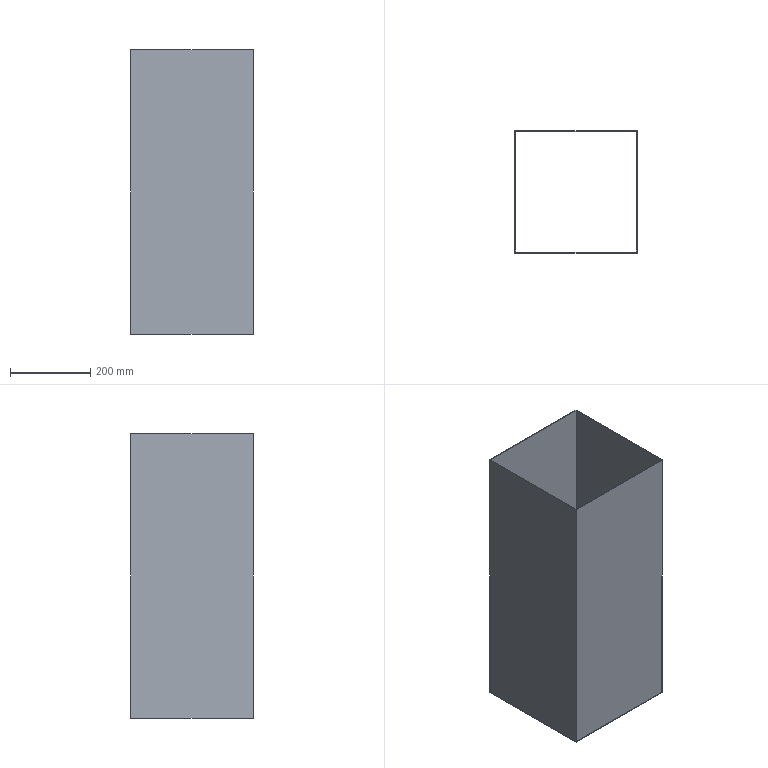Part | STEP file | Backup 2012-3-22-011 | 1 solid | 10 faces | box 304 x 304 x 708.25 mm | volume 1711132 mm3 | plane 10
STEP:
#1=CARTESIAN_POINT('',(0.,0.,0.));
#2=DIRECTION('',(0.,0.,1.));
#3=DIRECTION('',(1.,0.,0.));
#4=AXIS2_PLACEMENT_3D('',#1,#2,#3);
#5=CARTESIAN_POINT('',(-2.,2.,708.25));
#6=VERTEX_POINT('',#5);
#7=CARTESIAN_POINT('',(-2.,-302.,708.25));
#8=VERTEX_POINT('',#7);
#9=CARTESIAN_POINT('',(-2.,2.,708.25));
#10=DIRECTION('',(0.,-1.,0.));
#11=VECTOR('',#10,1.);
#12=LINE('',#9,#11);
#13=CARTESIAN_POINT('',(-2.,-302.,708.25));
#14=DIRECTION('',(0.,0.,1.));
#15=DIRECTION('',(1.,0.,0.));
#16=AXIS2_PLACEMENT_3D('',#13,#14,#15);
#17=PLANE('',#16);
#18=CARTESIAN_POINT('',(0.,304.));
#19=DIRECTION('',(0.,-1.));
#20=VECTOR('',#19,1.);
#21=LINE('',#18,#20);
#22=(GEOMETRIC_REPRESENTATION_CONTEXT(2)PARAMETRIC_REPRESENTATION_CONTEXT()REPRESENTATION_CONTEXT('',''));
#23=DEFINITIONAL_REPRESENTATION('',(#21),#22);
#24=PCURVE('',#17,#23);
#25=CARTESIAN_POINT('',(-2.,2.,708.25));
#26=DIRECTION('',(1.,0.,0.));
#27=DIRECTION('',(0.,1.,0.));
#28=AXIS2_PLACEMENT_3D('',#25,#26,#27);
#29=PLANE('',#28);
#30=CARTESIAN_POINT('',(0.,0.));
#31=DIRECTION('',(-1.,0.));
#32=VECTOR('',#31,1.);
#33=LINE('',#30,#32);
#34=(GEOMETRIC_REPRESENTATION_CONTEXT(2)PARAMETRIC_REPRESENTATION_CONTEXT()REPRESENTATION_CONTEXT('',''));
#35=DEFINITIONAL_REPRESENTATION('',(#33),#34);
#36=PCURVE('',#29,#35);
#37=SURFACE_CURVE('',#12,(#24,#36),.PCURVE_S1.);
#38=EDGE_CURVE('',#6,#8,#37,.T.);
#39=ORIENTED_EDGE('',*,*,#38,.T.);
#40=CARTESIAN_POINT('',(302.,-302.,708.25));
#41=VERTEX_POINT('',#40);
#42=CARTESIAN_POINT('',(-2.,-302.,708.25));
#43=DIRECTION('',(1.,0.,0.));
#44=VECTOR('',#43,1.);
#45=LINE('',#42,#44);
#46=CARTESIAN_POINT('',(0.,0.));
#47=DIRECTION('',(1.,0.));
#48=VECTOR('',#47,1.);
#49=LINE('',#46,#48);
#50=(GEOMETRIC_REPRESENTATION_CONTEXT(2)PARAMETRIC_REPRESENTATION_CONTEXT()REPRESENTATION_CONTEXT('',''));
#51=DEFINITIONAL_REPRESENTATION('',(#49),#50);
#52=PCURVE('',#17,#51);
#53=CARTESIAN_POINT('',(-2.,-302.,708.25));
#54=DIRECTION('',(0.,1.,0.));
#55=DIRECTION('',(0.,0.,1.));
#56=AXIS2_PLACEMENT_3D('',#53,#54,#55);
#57=PLANE('',#56);
#58=CARTESIAN_POINT('',(0.,0.));
#59=DIRECTION('',(0.,1.));
#60=VECTOR('',#59,1.);
#61=LINE('',#58,#60);
#62=(GEOMETRIC_REPRESENTATION_CONTEXT(2)PARAMETRIC_REPRESENTATION_CONTEXT()REPRESENTATION_CONTEXT('',''));
#63=DEFINITIONAL_REPRESENTATION('',(#61),#62);
#64=PCURVE('',#57,#63);
#65=SURFACE_CURVE('',#45,(#52,#64),.PCURVE_S1.);
#66=EDGE_CURVE('',#8,#41,#65,.T.);
#67=ORIENTED_EDGE('',*,*,#66,.T.);
#68=CARTESIAN_POINT('',(302.,2.,708.25));
#69=VERTEX_POINT('',#68);
#70=CARTESIAN_POINT('',(302.,2.,708.25));
#71=DIRECTION('',(0.,1.,0.));
#72=VECTOR('',#71,1.);
#73=LINE('',#70,#72);
#74=CARTESIAN_POINT('',(304.,304.));
#75=DIRECTION('',(0.,1.));
#76=VECTOR('',#75,1.);
#77=LINE('',#74,#76);
#78=(GEOMETRIC_REPRESENTATION_CONTEXT(2)PARAMETRIC_REPRESENTATION_CONTEXT()REPRESENTATION_CONTEXT('',''));
#79=DEFINITIONAL_REPRESENTATION('',(#77),#78);
#80=PCURVE('',#17,#79);
#81=CARTESIAN_POINT('',(302.,2.,708.25));
#82=DIRECTION('',(-1.,0.,0.));
#83=DIRECTION('',(0.,-1.,0.));
#84=AXIS2_PLACEMENT_3D('',#81,#82,#83);
#85=PLANE('',#84);
#86=CARTESIAN_POINT('',(0.,0.));
#87=DIRECTION('',(-1.,0.));
#88=VECTOR('',#87,1.);
#89=LINE('',#86,#88);
#90=(GEOMETRIC_REPRESENTATION_CONTEXT(2)PARAMETRIC_REPRESENTATION_CONTEXT()REPRESENTATION_CONTEXT('',''));
#91=DEFINITIONAL_REPRESENTATION('',(#89),#90);
#92=PCURVE('',#85,#91);
#93=SURFACE_CURVE('',#73,(#80,#92),.PCURVE_S1.);
#94=EDGE_CURVE('',#41,#69,#93,.T.);
#95=ORIENTED_EDGE('',*,*,#94,.T.);
#96=CARTESIAN_POINT('',(-2.,2.,708.25));
#97=DIRECTION('',(-1.,0.,0.));
#98=VECTOR('',#97,1.);
#99=LINE('',#96,#98);
#100=CARTESIAN_POINT('',(0.,304.));
#101=DIRECTION('',(-1.,0.));
#102=VECTOR('',#101,1.);
#103=LINE('',#100,#102);
#104=(GEOMETRIC_REPRESENTATION_CONTEXT(2)PARAMETRIC_REPRESENTATION_CONTEXT()REPRESENTATION_CONTEXT('',''));
#105=DEFINITIONAL_REPRESENTATION('',(#103),#104);
#106=PCURVE('',#17,#105);
#107=CARTESIAN_POINT('',(-2.,2.,708.25));
#108=DIRECTION('',(0.,-1.,0.));
#109=DIRECTION('',(0.,0.,-1.));
#110=AXIS2_PLACEMENT_3D('',#107,#108,#109);
#111=PLANE('',#110);
#112=CARTESIAN_POINT('',(0.,0.));
#113=DIRECTION('',(0.,-1.));
#114=VECTOR('',#113,1.);
#115=LINE('',#112,#114);
#116=(GEOMETRIC_REPRESENTATION_CONTEXT(2)PARAMETRIC_REPRESENTATION_CONTEXT()REPRESENTATION_CONTEXT('',''));
#117=DEFINITIONAL_REPRESENTATION('',(#115),#116);
#118=PCURVE('',#111,#117);
#119=SURFACE_CURVE('',#99,(#106,#118),.PCURVE_S1.);
#120=EDGE_CURVE('',#69,#6,#119,.T.);
#121=ORIENTED_EDGE('',*,*,#120,.T.);
#122=EDGE_LOOP('',(#39,#67,#95,#121));
#123=FACE_BOUND('',#122,.T.);
#124=CARTESIAN_POINT('',(0.,-300.,708.25));
#125=VERTEX_POINT('',#124);
#126=CARTESIAN_POINT('',(300.,-300.,708.25));
#127=VERTEX_POINT('',#126);
#128=CARTESIAN_POINT('',(0.,-300.,708.25));
#129=DIRECTION('',(1.,0.,0.));
#130=VECTOR('',#129,1.);
#131=LINE('',#128,#130);
#132=CARTESIAN_POINT('',(2.,2.));
#133=DIRECTION('',(1.,0.));
#134=VECTOR('',#133,1.);
#135=LINE('',#132,#134);
#136=(GEOMETRIC_REPRESENTATION_CONTEXT(2)PARAMETRIC_REPRESENTATION_CONTEXT()REPRESENTATION_CONTEXT('',''));
#137=DEFINITIONAL_REPRESENTATION('',(#135),#136);
#138=PCURVE('',#17,#137);
#139=CARTESIAN_POINT('',(0.,-300.,708.25));
#140=DIRECTION('',(0.,1.,0.));
#141=DIRECTION('',(0.,0.,1.));
#142=AXIS2_PLACEMENT_3D('',#139,#140,#141);
#143=PLANE('',#142);
#144=CARTESIAN_POINT('',(0.,0.));
#145=DIRECTION('',(0.,1.));
#146=VECTOR('',#145,1.);
#147=LINE('',#144,#146);
#148=(GEOMETRIC_REPRESENTATION_CONTEXT(2)PARAMETRIC_REPRESENTATION_CONTEXT()REPRESENTATION_CONTEXT('',''));
#149=DEFINITIONAL_REPRESENTATION('',(#147),#148);
#150=PCURVE('',#143,#149);
#151=SURFACE_CURVE('',#131,(#138,#150),.PCURVE_S1.);
#152=EDGE_CURVE('',#125,#127,#151,.T.);
#153=ORIENTED_EDGE('',*,*,#152,.F.);
#154=CARTESIAN_POINT('',(0.,0.,708.25));
#155=VERTEX_POINT('',#154);
#156=CARTESIAN_POINT('',(0.,0.,708.25));
#157=DIRECTION('',(0.,-1.,0.));
#158=VECTOR('',#157,1.);
#159=LINE('',#156,#158);
#160=CARTESIAN_POINT('',(2.,302.));
#161=DIRECTION('',(0.,-1.));
#162=VECTOR('',#161,1.);
#163=LINE('',#160,#162);
#164=(GEOMETRIC_REPRESENTATION_CONTEXT(2)PARAMETRIC_REPRESENTATION_CONTEXT()REPRESENTATION_CONTEXT('',''));
#165=DEFINITIONAL_REPRESENTATION('',(#163),#164);
#166=PCURVE('',#17,#165);
#167=CARTESIAN_POINT('',(0.,0.,708.25));
#168=DIRECTION('',(1.,0.,0.));
#169=DIRECTION('',(0.,1.,0.));
#170=AXIS2_PLACEMENT_3D('',#167,#168,#169);
#171=PLANE('',#170);
#172=CARTESIAN_POINT('',(0.,0.));
#173=DIRECTION('',(-1.,0.));
#174=VECTOR('',#173,1.);
#175=LINE('',#172,#174);
#176=(GEOMETRIC_REPRESENTATION_CONTEXT(2)PARAMETRIC_REPRESENTATION_CONTEXT()REPRESENTATION_CONTEXT('',''));
#177=DEFINITIONAL_REPRESENTATION('',(#175),#176);
#178=PCURVE('',#171,#177);
#179=SURFACE_CURVE('',#159,(#166,#178),.PCURVE_S1.);
#180=EDGE_CURVE('',#155,#125,#179,.T.);
#181=ORIENTED_EDGE('',*,*,#180,.F.);
#182=CARTESIAN_POINT('',(300.,0.,708.25));
#183=VERTEX_POINT('',#182);
#184=CARTESIAN_POINT('',(0.,0.,708.25));
#185=DIRECTION('',(-1.,0.,0.));
#186=VECTOR('',#185,1.);
#187=LINE('',#184,#186);
#188=CARTESIAN_POINT('',(2.,302.));
#189=DIRECTION('',(-1.,0.));
#190=VECTOR('',#189,1.);
#191=LINE('',#188,#190);
#192=(GEOMETRIC_REPRESENTATION_CONTEXT(2)PARAMETRIC_REPRESENTATION_CONTEXT()REPRESENTATION_CONTEXT('',''));
#193=DEFINITIONAL_REPRESENTATION('',(#191),#192);
#194=PCURVE('',#17,#193);
#195=CARTESIAN_POINT('',(0.,0.,708.25));
#196=DIRECTION('',(0.,-1.,0.));
#197=DIRECTION('',(0.,0.,-1.));
#198=AXIS2_PLACEMENT_3D('',#195,#196,#197);
#199=PLANE('',#198);
#200=CARTESIAN_POINT('',(0.,0.));
#201=DIRECTION('',(0.,-1.));
#202=VECTOR('',#201,1.);
#203=LINE('',#200,#202);
#204=(GEOMETRIC_REPRESENTATION_CONTEXT(2)PARAMETRIC_REPRESENTATION_CONTEXT()REPRESENTATION_CONTEXT('',''));
#205=DEFINITIONAL_REPRESENTATION('',(#203),#204);
#206=PCURVE('',#199,#205);
#207=SURFACE_CURVE('',#187,(#194,#206),.PCURVE_S1.);
#208=EDGE_CURVE('',#183,#155,#207,.T.);
#209=ORIENTED_EDGE('',*,*,#208,.F.);
#210=CARTESIAN_POINT('',(300.,0.,708.25));
#211=DIRECTION('',(0.,1.,0.));
#212=VECTOR('',#211,1.);
#213=LINE('',#210,#212);
#214=CARTESIAN_POINT('',(302.,302.));
#215=DIRECTION('',(0.,1.));
#216=VECTOR('',#215,1.);
#217=LINE('',#214,#216);
#218=(GEOMETRIC_REPRESENTATION_CONTEXT(2)PARAMETRIC_REPRESENTATION_CONTEXT()REPRESENTATION_CONTEXT('',''));
#219=DEFINITIONAL_REPRESENTATION('',(#217),#218);
#220=PCURVE('',#17,#219);
#221=CARTESIAN_POINT('',(300.,0.,708.25));
#222=DIRECTION('',(-1.,0.,0.));
#223=DIRECTION('',(0.,-1.,0.));
#224=AXIS2_PLACEMENT_3D('',#221,#222,#223);
#225=PLANE('',#224);
#226=CARTESIAN_POINT('',(0.,0.));
#227=DIRECTION('',(-1.,0.));
#228=VECTOR('',#227,1.);
#229=LINE('',#226,#228);
#230=(GEOMETRIC_REPRESENTATION_CONTEXT(2)PARAMETRIC_REPRESENTATION_CONTEXT()REPRESENTATION_CONTEXT('',''));
#231=DEFINITIONAL_REPRESENTATION('',(#229),#230);
#232=PCURVE('',#225,#231);
#233=SURFACE_CURVE('',#213,(#220,#232),.PCURVE_S1.);
#234=EDGE_CURVE('',#127,#183,#233,.T.);
#235=ORIENTED_EDGE('',*,*,#234,.F.);
#236=EDGE_LOOP('',(#153,#181,#209,#235));
#237=FACE_BOUND('',#236,.T.);
#238=ADVANCED_FACE('',(#123,#237),#17,.T.);
#239=CARTESIAN_POINT('',(-2.,2.,0.));
#240=VERTEX_POINT('',#239);
#241=CARTESIAN_POINT('',(-2.,-302.,0.));
#242=VERTEX_POINT('',#241);
#243=CARTESIAN_POINT('',(-2.,2.,0.));
#244=DIRECTION('',(0.,-1.,0.));
#245=VECTOR('',#244,1.);
#246=LINE('',#243,#245);
#247=CARTESIAN_POINT('',(-2.,-302.,0.));
#248=DIRECTION('',(0.,0.,1.));
#249=DIRECTION('',(1.,0.,0.));
#250=AXIS2_PLACEMENT_3D('',#247,#248,#249);
#251=PLANE('',#250);
#252=CARTESIAN_POINT('',(0.,304.));
#253=DIRECTION('',(0.,-1.));
#254=VECTOR('',#253,1.);
#255=LINE('',#252,#254);
#256=(GEOMETRIC_REPRESENTATION_CONTEXT(2)PARAMETRIC_REPRESENTATION_CONTEXT()REPRESENTATION_CONTEXT('',''));
#257=DEFINITIONAL_REPRESENTATION('',(#255),#256);
#258=PCURVE('',#251,#257);
#259=CARTESIAN_POINT('',(0.,-708.25));
#260=DIRECTION('',(-1.,0.));
#261=VECTOR('',#260,1.);
#262=LINE('',#259,#261);
#263=(GEOMETRIC_REPRESENTATION_CONTEXT(2)PARAMETRIC_REPRESENTATION_CONTEXT()REPRESENTATION_CONTEXT('',''));
#264=DEFINITIONAL_REPRESENTATION('',(#262),#263);
#265=PCURVE('',#29,#264);
#266=SURFACE_CURVE('',#246,(#258,#265),.PCURVE_S1.);
#267=EDGE_CURVE('',#240,#242,#266,.T.);
#268=ORIENTED_EDGE('',*,*,#267,.F.);
#269=CARTESIAN_POINT('',(302.,2.,0.));
#270=VERTEX_POINT('',#269);
#271=CARTESIAN_POINT('',(-2.,2.,0.));
#272=DIRECTION('',(-1.,0.,0.));
#273=VECTOR('',#272,1.);
#274=LINE('',#271,#273);
#275=CARTESIAN_POINT('',(0.,304.));
#276=DIRECTION('',(-1.,0.));
#277=VECTOR('',#276,1.);
#278=LINE('',#275,#277);
#279=(GEOMETRIC_REPRESENTATION_CONTEXT(2)PARAMETRIC_REPRESENTATION_CONTEXT()REPRESENTATION_CONTEXT('',''));
#280=DEFINITIONAL_REPRESENTATION('',(#278),#279);
#281=PCURVE('',#251,#280);
#282=CARTESIAN_POINT('',(708.25,0.));
#283=DIRECTION('',(0.,-1.));
#284=VECTOR('',#283,1.);
#285=LINE('',#282,#284);
#286=(GEOMETRIC_REPRESENTATION_CONTEXT(2)PARAMETRIC_REPRESENTATION_CONTEXT()REPRESENTATION_CONTEXT('',''));
#287=DEFINITIONAL_REPRESENTATION('',(#285),#286);
#288=PCURVE('',#111,#287);
#289=SURFACE_CURVE('',#274,(#281,#288),.PCURVE_S1.);
#290=EDGE_CURVE('',#270,#240,#289,.T.);
#291=ORIENTED_EDGE('',*,*,#290,.F.);
#292=CARTESIAN_POINT('',(302.,-302.,0.));
#293=VERTEX_POINT('',#292);
#294=CARTESIAN_POINT('',(302.,2.,0.));
#295=DIRECTION('',(0.,1.,0.));
#296=VECTOR('',#295,1.);
#297=LINE('',#294,#296);
#298=CARTESIAN_POINT('',(304.,304.));
#299=DIRECTION('',(0.,1.));
#300=VECTOR('',#299,1.);
#301=LINE('',#298,#300);
#302=(GEOMETRIC_REPRESENTATION_CONTEXT(2)PARAMETRIC_REPRESENTATION_CONTEXT()REPRESENTATION_CONTEXT('',''));
#303=DEFINITIONAL_REPRESENTATION('',(#301),#302);
#304=PCURVE('',#251,#303);
#305=CARTESIAN_POINT('',(0.,-708.25));
#306=DIRECTION('',(-1.,0.));
#307=VECTOR('',#306,1.);
#308=LINE('',#305,#307);
#309=(GEOMETRIC_REPRESENTATION_CONTEXT(2)PARAMETRIC_REPRESENTATION_CONTEXT()REPRESENTATION_CONTEXT('',''));
#310=DEFINITIONAL_REPRESENTATION('',(#308),#309);
#311=PCURVE('',#85,#310);
#312=SURFACE_CURVE('',#297,(#304,#311),.PCURVE_S1.);
#313=EDGE_CURVE('',#293,#270,#312,.T.);
#314=ORIENTED_EDGE('',*,*,#313,.F.);
#315=CARTESIAN_POINT('',(-2.,-302.,0.));
#316=DIRECTION('',(1.,0.,0.));
#317=VECTOR('',#316,1.);
#318=LINE('',#315,#317);
#319=CARTESIAN_POINT('',(0.,0.));
#320=DIRECTION('',(1.,0.));
#321=VECTOR('',#320,1.);
#322=LINE('',#319,#321);
#323=(GEOMETRIC_REPRESENTATION_CONTEXT(2)PARAMETRIC_REPRESENTATION_CONTEXT()REPRESENTATION_CONTEXT('',''));
#324=DEFINITIONAL_REPRESENTATION('',(#322),#323);
#325=PCURVE('',#251,#324);
#326=CARTESIAN_POINT('',(-708.25,0.));
#327=DIRECTION('',(0.,1.));
#328=VECTOR('',#327,1.);
#329=LINE('',#326,#328);
#330=(GEOMETRIC_REPRESENTATION_CONTEXT(2)PARAMETRIC_REPRESENTATION_CONTEXT()REPRESENTATION_CONTEXT('',''));
#331=DEFINITIONAL_REPRESENTATION('',(#329),#330);
#332=PCURVE('',#57,#331);
#333=SURFACE_CURVE('',#318,(#325,#332),.PCURVE_S1.);
#334=EDGE_CURVE('',#242,#293,#333,.T.);
#335=ORIENTED_EDGE('',*,*,#334,.F.);
#336=EDGE_LOOP('',(#268,#291,#314,#335));
#337=FACE_BOUND('',#336,.T.);
#338=CARTESIAN_POINT('',(0.,0.,0.));
#339=VERTEX_POINT('',#338);
#340=CARTESIAN_POINT('',(0.,-300.,0.));
#341=VERTEX_POINT('',#340);
#342=CARTESIAN_POINT('',(0.,0.,0.));
#343=DIRECTION('',(0.,-1.,0.));
#344=VECTOR('',#343,1.);
#345=LINE('',#342,#344);
#346=CARTESIAN_POINT('',(2.,302.));
#347=DIRECTION('',(0.,-1.));
#348=VECTOR('',#347,1.);
#349=LINE('',#346,#348);
#350=(GEOMETRIC_REPRESENTATION_CONTEXT(2)PARAMETRIC_REPRESENTATION_CONTEXT()REPRESENTATION_CONTEXT('',''));
#351=DEFINITIONAL_REPRESENTATION('',(#349),#350);
#352=PCURVE('',#251,#351);
#353=CARTESIAN_POINT('',(0.,-708.25));
#354=DIRECTION('',(-1.,0.));
#355=VECTOR('',#354,1.);
#356=LINE('',#353,#355);
#357=(GEOMETRIC_REPRESENTATION_CONTEXT(2)PARAMETRIC_REPRESENTATION_CONTEXT()REPRESENTATION_CONTEXT('',''));
#358=DEFINITIONAL_REPRESENTATION('',(#356),#357);
#359=PCURVE('',#171,#358);
#360=SURFACE_CURVE('',#345,(#352,#359),.PCURVE_S1.);
#361=EDGE_CURVE('',#339,#341,#360,.T.);
#362=ORIENTED_EDGE('',*,*,#361,.T.);
#363=CARTESIAN_POINT('',(300.,-300.,0.));
#364=VERTEX_POINT('',#363);
#365=CARTESIAN_POINT('',(0.,-300.,0.));
#366=DIRECTION('',(1.,0.,0.));
#367=VECTOR('',#366,1.);
#368=LINE('',#365,#367);
#369=CARTESIAN_POINT('',(2.,2.));
#370=DIRECTION('',(1.,0.));
#371=VECTOR('',#370,1.);
#372=LINE('',#369,#371);
#373=(GEOMETRIC_REPRESENTATION_CONTEXT(2)PARAMETRIC_REPRESENTATION_CONTEXT()REPRESENTATION_CONTEXT('',''));
#374=DEFINITIONAL_REPRESENTATION('',(#372),#373);
#375=PCURVE('',#251,#374);
#376=CARTESIAN_POINT('',(-708.25,0.));
#377=DIRECTION('',(0.,1.));
#378=VECTOR('',#377,1.);
#379=LINE('',#376,#378);
#380=(GEOMETRIC_REPRESENTATION_CONTEXT(2)PARAMETRIC_REPRESENTATION_CONTEXT()REPRESENTATION_CONTEXT('',''));
#381=DEFINITIONAL_REPRESENTATION('',(#379),#380);
#382=PCURVE('',#143,#381);
#383=SURFACE_CURVE('',#368,(#375,#382),.PCURVE_S1.);
#384=EDGE_CURVE('',#341,#364,#383,.T.);
#385=ORIENTED_EDGE('',*,*,#384,.T.);
#386=CARTESIAN_POINT('',(300.,0.,0.));
#387=VERTEX_POINT('',#386);
#388=CARTESIAN_POINT('',(300.,0.,0.));
#389=DIRECTION('',(0.,1.,0.));
#390=VECTOR('',#389,1.);
#391=LINE('',#388,#390);
#392=CARTESIAN_POINT('',(302.,302.));
#393=DIRECTION('',(0.,1.));
#394=VECTOR('',#393,1.);
#395=LINE('',#392,#394);
#396=(GEOMETRIC_REPRESENTATION_CONTEXT(2)PARAMETRIC_REPRESENTATION_CONTEXT()REPRESENTATION_CONTEXT('',''));
#397=DEFINITIONAL_REPRESENTATION('',(#395),#396);
#398=PCURVE('',#251,#397);
#399=CARTESIAN_POINT('',(0.,-708.25));
#400=DIRECTION('',(-1.,0.));
#401=VECTOR('',#400,1.);
#402=LINE('',#399,#401);
#403=(GEOMETRIC_REPRESENTATION_CONTEXT(2)PARAMETRIC_REPRESENTATION_CONTEXT()REPRESENTATION_CONTEXT('',''));
#404=DEFINITIONAL_REPRESENTATION('',(#402),#403);
#405=PCURVE('',#225,#404);
#406=SURFACE_CURVE('',#391,(#398,#405),.PCURVE_S1.);
#407=EDGE_CURVE('',#364,#387,#406,.T.);
#408=ORIENTED_EDGE('',*,*,#407,.T.);
#409=CARTESIAN_POINT('',(0.,0.,0.));
#410=DIRECTION('',(-1.,0.,0.));
#411=VECTOR('',#410,1.);
#412=LINE('',#409,#411);
#413=CARTESIAN_POINT('',(2.,302.));
#414=DIRECTION('',(-1.,0.));
#415=VECTOR('',#414,1.);
#416=LINE('',#413,#415);
#417=(GEOMETRIC_REPRESENTATION_CONTEXT(2)PARAMETRIC_REPRESENTATION_CONTEXT()REPRESENTATION_CONTEXT('',''));
#418=DEFINITIONAL_REPRESENTATION('',(#416),#417);
#419=PCURVE('',#251,#418);
#420=CARTESIAN_POINT('',(708.25,0.));
#421=DIRECTION('',(0.,-1.));
#422=VECTOR('',#421,1.);
#423=LINE('',#420,#422);
#424=(GEOMETRIC_REPRESENTATION_CONTEXT(2)PARAMETRIC_REPRESENTATION_CONTEXT()REPRESENTATION_CONTEXT('',''));
#425=DEFINITIONAL_REPRESENTATION('',(#423),#424);
#426=PCURVE('',#199,#425);
#427=SURFACE_CURVE('',#412,(#419,#426),.PCURVE_S1.);
#428=EDGE_CURVE('',#387,#339,#427,.T.);
#429=ORIENTED_EDGE('',*,*,#428,.T.);
#430=EDGE_LOOP('',(#362,#385,#408,#429));
#431=FACE_BOUND('',#430,.T.);
#432=ADVANCED_FACE('',(#337,#431),#251,.F.);
#433=ORIENTED_EDGE('',*,*,#267,.T.);
#434=CARTESIAN_POINT('',(-2.,-302.,708.25));
#435=DIRECTION('',(0.,0.,-1.));
#436=VECTOR('',#435,1.);
#437=LINE('',#434,#436);
#438=CARTESIAN_POINT('',(-304.,0.));
#439=DIRECTION('',(0.,-1.));
#440=VECTOR('',#439,1.);
#441=LINE('',#438,#440);
#442=(GEOMETRIC_REPRESENTATION_CONTEXT(2)PARAMETRIC_REPRESENTATION_CONTEXT()REPRESENTATION_CONTEXT('',''));
#443=DEFINITIONAL_REPRESENTATION('',(#441),#442);
#444=PCURVE('',#29,#443);
#445=CARTESIAN_POINT('',(0.,0.));
#446=DIRECTION('',(-1.,0.));
#447=VECTOR('',#446,1.);
#448=LINE('',#445,#447);
#449=(GEOMETRIC_REPRESENTATION_CONTEXT(2)PARAMETRIC_REPRESENTATION_CONTEXT()REPRESENTATION_CONTEXT('',''));
#450=DEFINITIONAL_REPRESENTATION('',(#448),#449);
#451=PCURVE('',#57,#450);
#452=SURFACE_CURVE('',#437,(#444,#451),.PCURVE_S1.);
#453=EDGE_CURVE('',#8,#242,#452,.T.);
#454=ORIENTED_EDGE('',*,*,#453,.F.);
#455=ORIENTED_EDGE('',*,*,#38,.F.);
#456=CARTESIAN_POINT('',(-2.,2.,708.25));
#457=DIRECTION('',(0.,0.,-1.));
#458=VECTOR('',#457,1.);
#459=LINE('',#456,#458);
#460=CARTESIAN_POINT('',(0.,0.));
#461=DIRECTION('',(0.,-1.));
#462=VECTOR('',#461,1.);
#463=LINE('',#460,#462);
#464=(GEOMETRIC_REPRESENTATION_CONTEXT(2)PARAMETRIC_REPRESENTATION_CONTEXT()REPRESENTATION_CONTEXT('',''));
#465=DEFINITIONAL_REPRESENTATION('',(#463),#464);
#466=PCURVE('',#29,#465);
#467=CARTESIAN_POINT('',(0.,0.));
#468=DIRECTION('',(1.,0.));
#469=VECTOR('',#468,1.);
#470=LINE('',#467,#469);
#471=(GEOMETRIC_REPRESENTATION_CONTEXT(2)PARAMETRIC_REPRESENTATION_CONTEXT()REPRESENTATION_CONTEXT('',''));
#472=DEFINITIONAL_REPRESENTATION('',(#470),#471);
#473=PCURVE('',#111,#472);
#474=SURFACE_CURVE('',#459,(#466,#473),.PCURVE_S1.);
#475=EDGE_CURVE('',#6,#240,#474,.T.);
#476=ORIENTED_EDGE('',*,*,#475,.T.);
#477=EDGE_LOOP('',(#433,#454,#455,#476));
#478=FACE_BOUND('',#477,.T.);
#479=ADVANCED_FACE('',(#478),#29,.F.);
#480=ORIENTED_EDGE('',*,*,#334,.T.);
#481=CARTESIAN_POINT('',(302.,-302.,708.25));
#482=DIRECTION('',(0.,0.,-1.));
#483=VECTOR('',#482,1.);
#484=LINE('',#481,#483);
#485=CARTESIAN_POINT('',(0.,304.));
#486=DIRECTION('',(-1.,0.));
#487=VECTOR('',#486,1.);
#488=LINE('',#485,#487);
#489=(GEOMETRIC_REPRESENTATION_CONTEXT(2)PARAMETRIC_REPRESENTATION_CONTEXT()REPRESENTATION_CONTEXT('',''));
#490=DEFINITIONAL_REPRESENTATION('',(#488),#489);
#491=PCURVE('',#57,#490);
#492=CARTESIAN_POINT('',(304.,0.));
#493=DIRECTION('',(0.,-1.));
#494=VECTOR('',#493,1.);
#495=LINE('',#492,#494);
#496=(GEOMETRIC_REPRESENTATION_CONTEXT(2)PARAMETRIC_REPRESENTATION_CONTEXT()REPRESENTATION_CONTEXT('',''));
#497=DEFINITIONAL_REPRESENTATION('',(#495),#496);
#498=PCURVE('',#85,#497);
#499=SURFACE_CURVE('',#484,(#491,#498),.PCURVE_S1.);
#500=EDGE_CURVE('',#41,#293,#499,.T.);
#501=ORIENTED_EDGE('',*,*,#500,.F.);
#502=ORIENTED_EDGE('',*,*,#66,.F.);
#503=ORIENTED_EDGE('',*,*,#453,.T.);
#504=EDGE_LOOP('',(#480,#501,#502,#503));
#505=FACE_BOUND('',#504,.T.);
#506=ADVANCED_FACE('',(#505),#57,.F.);
#507=ORIENTED_EDGE('',*,*,#313,.T.);
#508=CARTESIAN_POINT('',(302.,2.,708.25));
#509=DIRECTION('',(0.,0.,-1.));
#510=VECTOR('',#509,1.);
#511=LINE('',#508,#510);
#512=CARTESIAN_POINT('',(0.,0.));
#513=DIRECTION('',(0.,-1.));
#514=VECTOR('',#513,1.);
#515=LINE('',#512,#514);
#516=(GEOMETRIC_REPRESENTATION_CONTEXT(2)PARAMETRIC_REPRESENTATION_CONTEXT()REPRESENTATION_CONTEXT('',''));
#517=DEFINITIONAL_REPRESENTATION('',(#515),#516);
#518=PCURVE('',#85,#517);
#519=CARTESIAN_POINT('',(0.,304.));
#520=DIRECTION('',(1.,0.));
#521=VECTOR('',#520,1.);
#522=LINE('',#519,#521);
#523=(GEOMETRIC_REPRESENTATION_CONTEXT(2)PARAMETRIC_REPRESENTATION_CONTEXT()REPRESENTATION_CONTEXT('',''));
#524=DEFINITIONAL_REPRESENTATION('',(#522),#523);
#525=PCURVE('',#111,#524);
#526=SURFACE_CURVE('',#511,(#518,#525),.PCURVE_S1.);
#527=EDGE_CURVE('',#69,#270,#526,.T.);
#528=ORIENTED_EDGE('',*,*,#527,.F.);
#529=ORIENTED_EDGE('',*,*,#94,.F.);
#530=ORIENTED_EDGE('',*,*,#500,.T.);
#531=EDGE_LOOP('',(#507,#528,#529,#530));
#532=FACE_BOUND('',#531,.T.);
#533=ADVANCED_FACE('',(#532),#85,.F.);
#534=ORIENTED_EDGE('',*,*,#290,.T.);
#535=ORIENTED_EDGE('',*,*,#475,.F.);
#536=ORIENTED_EDGE('',*,*,#120,.F.);
#537=ORIENTED_EDGE('',*,*,#527,.T.);
#538=EDGE_LOOP('',(#534,#535,#536,#537));
#539=FACE_BOUND('',#538,.T.);
#540=ADVANCED_FACE('',(#539),#111,.F.);
#541=ORIENTED_EDGE('',*,*,#361,.F.);
#542=CARTESIAN_POINT('',(0.,0.,708.25));
#543=DIRECTION('',(0.,0.,-1.));
#544=VECTOR('',#543,1.);
#545=LINE('',#542,#544);
#546=CARTESIAN_POINT('',(0.,0.));
#547=DIRECTION('',(0.,-1.));
#548=VECTOR('',#547,1.);
#549=LINE('',#546,#548);
#550=(GEOMETRIC_REPRESENTATION_CONTEXT(2)PARAMETRIC_REPRESENTATION_CONTEXT()REPRESENTATION_CONTEXT('',''));
#551=DEFINITIONAL_REPRESENTATION('',(#549),#550);
#552=PCURVE('',#171,#551);
#553=CARTESIAN_POINT('',(0.,0.));
#554=DIRECTION('',(1.,0.));
#555=VECTOR('',#554,1.);
#556=LINE('',#553,#555);
#557=(GEOMETRIC_REPRESENTATION_CONTEXT(2)PARAMETRIC_REPRESENTATION_CONTEXT()REPRESENTATION_CONTEXT('',''));
#558=DEFINITIONAL_REPRESENTATION('',(#556),#557);
#559=PCURVE('',#199,#558);
#560=SURFACE_CURVE('',#545,(#552,#559),.PCURVE_S1.);
#561=EDGE_CURVE('',#155,#339,#560,.T.);
#562=ORIENTED_EDGE('',*,*,#561,.F.);
#563=ORIENTED_EDGE('',*,*,#180,.T.);
#564=CARTESIAN_POINT('',(0.,-300.,708.25));
#565=DIRECTION('',(0.,0.,-1.));
#566=VECTOR('',#565,1.);
#567=LINE('',#564,#566);
#568=CARTESIAN_POINT('',(-300.,0.));
#569=DIRECTION('',(0.,-1.));
#570=VECTOR('',#569,1.);
#571=LINE('',#568,#570);
#572=(GEOMETRIC_REPRESENTATION_CONTEXT(2)PARAMETRIC_REPRESENTATION_CONTEXT()REPRESENTATION_CONTEXT('',''));
#573=DEFINITIONAL_REPRESENTATION('',(#571),#572);
#574=PCURVE('',#171,#573);
#575=CARTESIAN_POINT('',(0.,0.));
#576=DIRECTION('',(-1.,0.));
#577=VECTOR('',#576,1.);
#578=LINE('',#575,#577);
#579=(GEOMETRIC_REPRESENTATION_CONTEXT(2)PARAMETRIC_REPRESENTATION_CONTEXT()REPRESENTATION_CONTEXT('',''));
#580=DEFINITIONAL_REPRESENTATION('',(#578),#579);
#581=PCURVE('',#143,#580);
#582=SURFACE_CURVE('',#567,(#574,#581),.PCURVE_S1.);
#583=EDGE_CURVE('',#125,#341,#582,.T.);
#584=ORIENTED_EDGE('',*,*,#583,.T.);
#585=EDGE_LOOP('',(#541,#562,#563,#584));
#586=FACE_BOUND('',#585,.T.);
#587=ADVANCED_FACE('',(#586),#171,.T.);
#588=ORIENTED_EDGE('',*,*,#384,.F.);
#589=ORIENTED_EDGE('',*,*,#583,.F.);
#590=ORIENTED_EDGE('',*,*,#152,.T.);
#591=CARTESIAN_POINT('',(300.,-300.,708.25));
#592=DIRECTION('',(0.,0.,-1.));
#593=VECTOR('',#592,1.);
#594=LINE('',#591,#593);
#595=CARTESIAN_POINT('',(0.,300.));
#596=DIRECTION('',(-1.,0.));
#597=VECTOR('',#596,1.);
#598=LINE('',#595,#597);
#599=(GEOMETRIC_REPRESENTATION_CONTEXT(2)PARAMETRIC_REPRESENTATION_CONTEXT()REPRESENTATION_CONTEXT('',''));
#600=DEFINITIONAL_REPRESENTATION('',(#598),#599);
#601=PCURVE('',#143,#600);
#602=CARTESIAN_POINT('',(300.,0.));
#603=DIRECTION('',(0.,-1.));
#604=VECTOR('',#603,1.);
#605=LINE('',#602,#604);
#606=(GEOMETRIC_REPRESENTATION_CONTEXT(2)PARAMETRIC_REPRESENTATION_CONTEXT()REPRESENTATION_CONTEXT('',''));
#607=DEFINITIONAL_REPRESENTATION('',(#605),#606);
#608=PCURVE('',#225,#607);
#609=SURFACE_CURVE('',#594,(#601,#608),.PCURVE_S1.);
#610=EDGE_CURVE('',#127,#364,#609,.T.);
#611=ORIENTED_EDGE('',*,*,#610,.T.);
#612=EDGE_LOOP('',(#588,#589,#590,#611));
#613=FACE_BOUND('',#612,.T.);
#614=ADVANCED_FACE('',(#613),#143,.T.);
#615=ORIENTED_EDGE('',*,*,#407,.F.);
#616=ORIENTED_EDGE('',*,*,#610,.F.);
#617=ORIENTED_EDGE('',*,*,#234,.T.);
#618=CARTESIAN_POINT('',(300.,0.,708.25));
#619=DIRECTION('',(0.,0.,-1.));
#620=VECTOR('',#619,1.);
#621=LINE('',#618,#620);
#622=CARTESIAN_POINT('',(0.,0.));
#623=DIRECTION('',(0.,-1.));
#624=VECTOR('',#623,1.);
#625=LINE('',#622,#624);
#626=(GEOMETRIC_REPRESENTATION_CONTEXT(2)PARAMETRIC_REPRESENTATION_CONTEXT()REPRESENTATION_CONTEXT('',''));
#627=DEFINITIONAL_REPRESENTATION('',(#625),#626);
#628=PCURVE('',#225,#627);
#629=CARTESIAN_POINT('',(0.,300.));
#630=DIRECTION('',(1.,0.));
#631=VECTOR('',#630,1.);
#632=LINE('',#629,#631);
#633=(GEOMETRIC_REPRESENTATION_CONTEXT(2)PARAMETRIC_REPRESENTATION_CONTEXT()REPRESENTATION_CONTEXT('',''));
#634=DEFINITIONAL_REPRESENTATION('',(#632),#633);
#635=PCURVE('',#199,#634);
#636=SURFACE_CURVE('',#621,(#628,#635),.PCURVE_S1.);
#637=EDGE_CURVE('',#183,#387,#636,.T.);
#638=ORIENTED_EDGE('',*,*,#637,.T.);
#639=EDGE_LOOP('',(#615,#616,#617,#638));
#640=FACE_BOUND('',#639,.T.);
#641=ADVANCED_FACE('',(#640),#225,.T.);
#642=ORIENTED_EDGE('',*,*,#428,.F.);
#643=ORIENTED_EDGE('',*,*,#637,.F.);
#644=ORIENTED_EDGE('',*,*,#208,.T.);
#645=ORIENTED_EDGE('',*,*,#561,.T.);
#646=EDGE_LOOP('',(#642,#643,#644,#645));
#647=FACE_BOUND('',#646,.T.);
#648=ADVANCED_FACE('',(#647),#199,.T.);
#649=CLOSED_SHELL('',(#238,#432,#479,#506,#533,#540,#587,#614,#641,#648));
#650=MANIFOLD_SOLID_BREP('',#649);
#651=(LENGTH_UNIT()NAMED_UNIT(*)SI_UNIT(.MILLI.,.METRE.));
#652=UNCERTAINTY_MEASURE_WITH_UNIT(LENGTH_MEASURE(0.0000001),#651,'','');
#653=(NAMED_UNIT(*)PLANE_ANGLE_UNIT()SI_UNIT($,.RADIAN.));
#654=(NAMED_UNIT(*)SI_UNIT($,.STERADIAN.)SOLID_ANGLE_UNIT());
#655=(GEOMETRIC_REPRESENTATION_CONTEXT(3)GLOBAL_UNCERTAINTY_ASSIGNED_CONTEXT((#652))GLOBAL_UNIT_ASSIGNED_CONTEXT((#651,#653,#654))REPRESENTATION_CONTEXT('',''));
#656=ADVANCED_BREP_SHAPE_REPRESENTATION('',(#4,#650),#655);